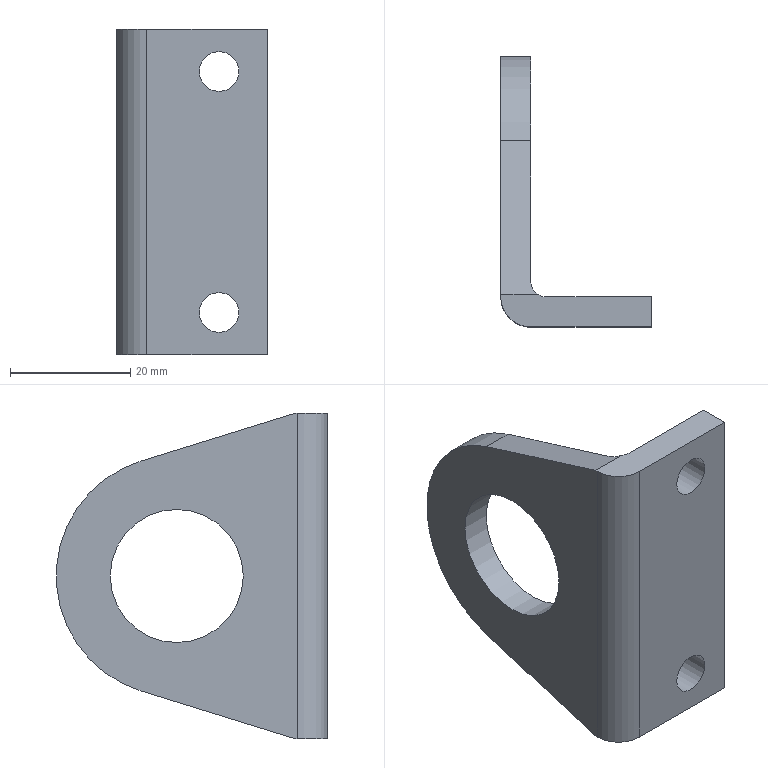Part | STEP file | 1_34 | 1 solid | 15 faces | box 25 x 45 x 54 mm | volume 12239 mm3 | plane 9 | cylinder 6 | commonest cylinder face diameters 6.6 x2 5 x1 10 x1 22.1 x1 40 x1
STEP:
#1=CARTESIAN_POINT('',(0.,0.,0.));
#2=DIRECTION('',(0.,0.,1.));
#3=DIRECTION('',(1.,0.,0.));
#4=AXIS2_PLACEMENT_3D('',#1,#2,#3);
#5=CARTESIAN_POINT('',(5.,25.,11.05));
#6=VERTEX_POINT('',#5);
#7=CARTESIAN_POINT('',(5.,25.,0.));
#8=DIRECTION('',(1.,0.,0.));
#9=DIRECTION('',(0.,1.,0.));
#10=AXIS2_PLACEMENT_3D('',#7,#8,#9);
#11=CIRCLE('',#10,11.05);
#12=CARTESIAN_POINT('',(5.1,25.,0.));
#13=DIRECTION('',(1.,0.,0.));
#14=DIRECTION('',(0.,0.,1.));
#15=AXIS2_PLACEMENT_3D('',#12,#13,#14);
#16=CYLINDRICAL_SURFACE('',#15,11.05);
#17=CARTESIAN_POINT('',(-1.571,-0.1));
#18=DIRECTION('',(1.,0.));
#19=VECTOR('',#18,1.);
#20=LINE('',#17,#19);
#21=(GEOMETRIC_REPRESENTATION_CONTEXT(2)PARAMETRIC_REPRESENTATION_CONTEXT()REPRESENTATION_CONTEXT('',''));
#22=DEFINITIONAL_REPRESENTATION('',(#20),#21);
#23=PCURVE('',#16,#22);
#24=CARTESIAN_POINT('',(5.,7.5,27.));
#25=DIRECTION('',(1.,0.,0.));
#26=DIRECTION('',(0.,0.,-1.));
#27=AXIS2_PLACEMENT_3D('',#24,#25,#26);
#28=PLANE('',#27);
#29=CARTESIAN_POINT('',(27.,17.5));
#30=DIRECTION('',(0.,1.));
#31=AXIS2_PLACEMENT_2D('',#29,#30);
#32=CIRCLE('',#31,11.05);
#33=(GEOMETRIC_REPRESENTATION_CONTEXT(2)PARAMETRIC_REPRESENTATION_CONTEXT()REPRESENTATION_CONTEXT('',''));
#34=DEFINITIONAL_REPRESENTATION('',(#32),#33);
#35=PCURVE('',#28,#34);
#36=SURFACE_CURVE('',#11,(#23,#35),.PCURVE_S1.);
#37=EDGE_CURVE('',#6,#6,#36,.T.);
#38=ORIENTED_EDGE('',*,*,#37,.F.);
#39=CARTESIAN_POINT('',(0.,25.,11.05));
#40=VERTEX_POINT('',#39);
#41=CARTESIAN_POINT('',(0.,25.,11.05));
#42=CARTESIAN_POINT('',(5.,25.,11.05));
#43=B_SPLINE_CURVE_WITH_KNOTS('',1,(#41,#42),.UNSPECIFIED.,.F.,.F.,(2,2),(-5.1,-0.1),.PIECEWISE_BEZIER_KNOTS.);
#44=CARTESIAN_POINT('',(0.,0.));
#45=DIRECTION('',(0.,1.));
#46=VECTOR('',#45,1.);
#47=LINE('',#44,#46);
#48=(GEOMETRIC_REPRESENTATION_CONTEXT(2)PARAMETRIC_REPRESENTATION_CONTEXT()REPRESENTATION_CONTEXT('',''));
#49=DEFINITIONAL_REPRESENTATION('',(#47),#48);
#50=PCURVE('',#16,#49);
#51=CARTESIAN_POINT('',(6.283,0.));
#52=DIRECTION('',(0.,1.));
#53=VECTOR('',#52,1.);
#54=LINE('',#51,#53);
#55=(GEOMETRIC_REPRESENTATION_CONTEXT(2)PARAMETRIC_REPRESENTATION_CONTEXT()REPRESENTATION_CONTEXT('',''));
#56=DEFINITIONAL_REPRESENTATION('',(#54),#55);
#57=PCURVE('',#16,#56);
#58=SEAM_CURVE('',#43,(#50,#57),.PCURVE_S1.);
#59=EDGE_CURVE('',#40,#6,#58,.T.);
#60=ORIENTED_EDGE('',*,*,#59,.F.);
#61=CARTESIAN_POINT('',(0.,25.,0.));
#62=DIRECTION('',(1.,0.,0.));
#63=DIRECTION('',(0.,0.,-1.));
#64=AXIS2_PLACEMENT_3D('',#61,#62,#63);
#65=CIRCLE('',#64,11.05);
#66=CARTESIAN_POINT('',(-3.142,-5.1));
#67=DIRECTION('',(1.,0.));
#68=VECTOR('',#67,1.);
#69=LINE('',#66,#68);
#70=(GEOMETRIC_REPRESENTATION_CONTEXT(2)PARAMETRIC_REPRESENTATION_CONTEXT()REPRESENTATION_CONTEXT('',''));
#71=DEFINITIONAL_REPRESENTATION('',(#69),#70);
#72=PCURVE('',#16,#71);
#73=CARTESIAN_POINT('',(0.,50.,27.));
#74=DIRECTION('',(-1.,0.,0.));
#75=DIRECTION('',(0.,0.,1.));
#76=AXIS2_PLACEMENT_3D('',#73,#74,#75);
#77=PLANE('',#76);
#78=CARTESIAN_POINT('',(-38.05,-25.));
#79=CARTESIAN_POINT('',(-38.05,-5.861));
#80=CARTESIAN_POINT('',(-21.475,-15.43));
#81=CARTESIAN_POINT('',(-4.9,-25.));
#82=CARTESIAN_POINT('',(-21.475,-34.57));
#83=CARTESIAN_POINT('',(-38.05,-44.139));
#84=CARTESIAN_POINT('',(-38.05,-25.));
#85=(BOUNDED_CURVE()B_SPLINE_CURVE(2,(#78,#79,#80,#81,#82,#83,#84),.UNSPECIFIED.,.T.,.F.)B_SPLINE_CURVE_WITH_KNOTS((1,2,2,2,2,1),(-2.094,0.,2.094,4.189,6.283,8.378),.UNSPECIFIED.)CURVE()GEOMETRIC_REPRESENTATION_ITEM()RATIONAL_B_SPLINE_CURVE((1.,0.5,1.,0.5,1.,0.5,1.))REPRESENTATION_ITEM(''));
#86=(GEOMETRIC_REPRESENTATION_CONTEXT(2)PARAMETRIC_REPRESENTATION_CONTEXT()REPRESENTATION_CONTEXT('',''));
#87=DEFINITIONAL_REPRESENTATION('',(#85),#86);
#88=PCURVE('',#77,#87);
#89=SURFACE_CURVE('',#65,(#72,#88),.PCURVE_S1.);
#90=EDGE_CURVE('',#40,#40,#89,.T.);
#91=ORIENTED_EDGE('',*,*,#90,.T.);
#92=ORIENTED_EDGE('',*,*,#59,.T.);
#93=EDGE_LOOP('',(#38,#60,#91,#92));
#94=FACE_BOUND('',#93,.F.);
#95=ADVANCED_FACE('',(#94),#16,.F.);
#96=CARTESIAN_POINT('',(0.,5.423,27.));
#97=VERTEX_POINT('',#96);
#98=CARTESIAN_POINT('',(0.,30.917,19.105));
#99=VERTEX_POINT('',#98);
#100=CARTESIAN_POINT('',(0.,5.423,27.));
#101=DIRECTION('',(0.,0.9552,-0.2958));
#102=VECTOR('',#101,1.);
#103=LINE('',#100,#102);
#104=CARTESIAN_POINT('',(0.,-44.577));
#105=DIRECTION('',(-0.2958,0.9552));
#106=VECTOR('',#105,1.);
#107=LINE('',#104,#106);
#108=(GEOMETRIC_REPRESENTATION_CONTEXT(2)PARAMETRIC_REPRESENTATION_CONTEXT()REPRESENTATION_CONTEXT('',''));
#109=DEFINITIONAL_REPRESENTATION('',(#107),#108);
#110=PCURVE('',#77,#109);
#111=CARTESIAN_POINT('',(17.,-1.,28.989));
#112=DIRECTION('',(0.,-0.2958,-0.9552));
#113=DIRECTION('',(-1.,0.,0.));
#114=AXIS2_PLACEMENT_3D('',#111,#112,#113);
#115=PLANE('',#114);
#116=CARTESIAN_POINT('',(17.,6.724));
#117=DIRECTION('',(0.,1.));
#118=VECTOR('',#117,1.);
#119=LINE('',#116,#118);
#120=(GEOMETRIC_REPRESENTATION_CONTEXT(2)PARAMETRIC_REPRESENTATION_CONTEXT()REPRESENTATION_CONTEXT('',''));
#121=DEFINITIONAL_REPRESENTATION('',(#119),#120);
#122=PCURVE('',#115,#121);
#123=SURFACE_CURVE('',#103,(#110,#122),.PCURVE_S1.);
#124=EDGE_CURVE('',#97,#99,#123,.T.);
#125=ORIENTED_EDGE('',*,*,#124,.T.);
#126=CARTESIAN_POINT('',(0.,30.917,-19.105));
#127=VERTEX_POINT('',#126);
#128=CARTESIAN_POINT('',(0.,25.,0.));
#129=DIRECTION('',(-1.,0.,0.));
#130=DIRECTION('',(0.,1.,0.));
#131=AXIS2_PLACEMENT_3D('',#128,#129,#130);
#132=CIRCLE('',#131,20.);
#133=CARTESIAN_POINT('',(-27.,-25.));
#134=DIRECTION('',(0.,1.));
#135=AXIS2_PLACEMENT_2D('',#133,#134);
#136=CIRCLE('',#135,20.);
#137=(GEOMETRIC_REPRESENTATION_CONTEXT(2)PARAMETRIC_REPRESENTATION_CONTEXT()REPRESENTATION_CONTEXT('',''));
#138=DEFINITIONAL_REPRESENTATION('',(#136),#137);
#139=PCURVE('',#77,#138);
#140=CARTESIAN_POINT('',(17.,25.,0.));
#141=DIRECTION('',(1.,0.,0.));
#142=DIRECTION('',(0.,-0.2958,-0.9552));
#143=AXIS2_PLACEMENT_3D('',#140,#141,#142);
#144=CYLINDRICAL_SURFACE('',#143,20.);
#145=CARTESIAN_POINT('',(8.154,-17.));
#146=DIRECTION('',(-1.,0.));
#147=VECTOR('',#146,1.);
#148=LINE('',#145,#147);
#149=(GEOMETRIC_REPRESENTATION_CONTEXT(2)PARAMETRIC_REPRESENTATION_CONTEXT()REPRESENTATION_CONTEXT('',''));
#150=DEFINITIONAL_REPRESENTATION('',(#148),#149);
#151=PCURVE('',#144,#150);
#152=SURFACE_CURVE('',#132,(#139,#151),.PCURVE_S1.);
#153=EDGE_CURVE('',#99,#127,#152,.T.);
#154=ORIENTED_EDGE('',*,*,#153,.T.);
#155=CARTESIAN_POINT('',(0.,5.423,-27.));
#156=VERTEX_POINT('',#155);
#157=CARTESIAN_POINT('',(0.,30.917,-19.105));
#158=DIRECTION('',(0.,-0.9552,-0.2958));
#159=VECTOR('',#158,1.);
#160=LINE('',#157,#159);
#161=CARTESIAN_POINT('',(-46.105,-19.083));
#162=DIRECTION('',(-0.2958,-0.9552));
#163=VECTOR('',#162,1.);
#164=LINE('',#161,#163);
#165=(GEOMETRIC_REPRESENTATION_CONTEXT(2)PARAMETRIC_REPRESENTATION_CONTEXT()REPRESENTATION_CONTEXT('',''));
#166=DEFINITIONAL_REPRESENTATION('',(#164),#165);
#167=PCURVE('',#77,#166);
#168=CARTESIAN_POINT('',(17.,30.917,-19.105));
#169=DIRECTION('',(0.,-0.2958,0.9552));
#170=DIRECTION('',(1.,0.,0.));
#171=AXIS2_PLACEMENT_3D('',#168,#169,#170);
#172=PLANE('',#171);
#173=CARTESIAN_POINT('',(-17.,0.));
#174=DIRECTION('',(0.,-1.));
#175=VECTOR('',#174,1.);
#176=LINE('',#173,#175);
#177=(GEOMETRIC_REPRESENTATION_CONTEXT(2)PARAMETRIC_REPRESENTATION_CONTEXT()REPRESENTATION_CONTEXT('',''));
#178=DEFINITIONAL_REPRESENTATION('',(#176),#177);
#179=PCURVE('',#172,#178);
#180=SURFACE_CURVE('',#160,(#167,#179),.PCURVE_S1.);
#181=EDGE_CURVE('',#127,#156,#180,.T.);
#182=ORIENTED_EDGE('',*,*,#181,.T.);
#183=CARTESIAN_POINT('',(0.,5.,-27.));
#184=VERTEX_POINT('',#183);
#185=CARTESIAN_POINT('',(0.,5.423,-27.));
#186=DIRECTION('',(0.,-1.,0.));
#187=VECTOR('',#186,1.);
#188=LINE('',#185,#187);
#189=CARTESIAN_POINT('',(-54.,-44.577));
#190=DIRECTION('',(0.,-1.));
#191=VECTOR('',#190,1.);
#192=LINE('',#189,#191);
#193=(GEOMETRIC_REPRESENTATION_CONTEXT(2)PARAMETRIC_REPRESENTATION_CONTEXT()REPRESENTATION_CONTEXT('',''));
#194=DEFINITIONAL_REPRESENTATION('',(#192),#193);
#195=PCURVE('',#77,#194);
#196=CARTESIAN_POINT('',(0.,0.,-27.));
#197=DIRECTION('',(0.,0.,1.));
#198=DIRECTION('',(1.,0.,0.));
#199=AXIS2_PLACEMENT_3D('',#196,#197,#198);
#200=PLANE('',#199);
#201=CARTESIAN_POINT('',(0.,5.423));
#202=DIRECTION('',(0.,-1.));
#203=VECTOR('',#202,1.);
#204=LINE('',#201,#203);
#205=(GEOMETRIC_REPRESENTATION_CONTEXT(2)PARAMETRIC_REPRESENTATION_CONTEXT()REPRESENTATION_CONTEXT('',''));
#206=DEFINITIONAL_REPRESENTATION('',(#204),#205);
#207=PCURVE('',#200,#206);
#208=SURFACE_CURVE('',#188,(#195,#207),.PCURVE_S1.);
#209=EDGE_CURVE('',#156,#184,#208,.T.);
#210=ORIENTED_EDGE('',*,*,#209,.T.);
#211=CARTESIAN_POINT('',(0.,5.,27.));
#212=VERTEX_POINT('',#211);
#213=CARTESIAN_POINT('',(0.,5.,27.));
#214=DIRECTION('',(0.,0.,-1.));
#215=VECTOR('',#214,1.);
#216=LINE('',#213,#215);
#217=CARTESIAN_POINT('',(0.,-45.));
#218=DIRECTION('',(-1.,0.));
#219=VECTOR('',#218,1.);
#220=LINE('',#217,#219);
#221=(GEOMETRIC_REPRESENTATION_CONTEXT(2)PARAMETRIC_REPRESENTATION_CONTEXT()REPRESENTATION_CONTEXT('',''));
#222=DEFINITIONAL_REPRESENTATION('',(#220),#221);
#223=PCURVE('',#77,#222);
#224=CARTESIAN_POINT('',(5.,5.,27.));
#225=DIRECTION('',(0.,0.,1.));
#226=DIRECTION('',(-1.,0.,0.));
#227=AXIS2_PLACEMENT_3D('',#224,#225,#226);
#228=CYLINDRICAL_SURFACE('',#227,5.);
#229=CARTESIAN_POINT('',(0.,0.));
#230=DIRECTION('',(0.,-1.));
#231=VECTOR('',#230,1.);
#232=LINE('',#229,#231);
#233=(GEOMETRIC_REPRESENTATION_CONTEXT(2)PARAMETRIC_REPRESENTATION_CONTEXT()REPRESENTATION_CONTEXT('',''));
#234=DEFINITIONAL_REPRESENTATION('',(#232),#233);
#235=PCURVE('',#228,#234);
#236=SURFACE_CURVE('',#216,(#223,#235),.PCURVE_S1.);
#237=EDGE_CURVE('',#212,#184,#236,.T.);
#238=ORIENTED_EDGE('',*,*,#237,.F.);
#239=CARTESIAN_POINT('',(0.,5.423,27.));
#240=DIRECTION('',(0.,-1.,0.));
#241=VECTOR('',#240,1.);
#242=LINE('',#239,#241);
#243=CARTESIAN_POINT('',(0.,-44.577));
#244=DIRECTION('',(0.,-1.));
#245=VECTOR('',#244,1.);
#246=LINE('',#243,#245);
#247=(GEOMETRIC_REPRESENTATION_CONTEXT(2)PARAMETRIC_REPRESENTATION_CONTEXT()REPRESENTATION_CONTEXT('',''));
#248=DEFINITIONAL_REPRESENTATION('',(#246),#247);
#249=PCURVE('',#77,#248);
#250=CARTESIAN_POINT('',(0.,0.,27.));
#251=DIRECTION('',(0.,0.,1.));
#252=DIRECTION('',(1.,0.,0.));
#253=AXIS2_PLACEMENT_3D('',#250,#251,#252);
#254=PLANE('',#253);
#255=CARTESIAN_POINT('',(0.,5.423));
#256=DIRECTION('',(0.,-1.));
#257=VECTOR('',#256,1.);
#258=LINE('',#255,#257);
#259=(GEOMETRIC_REPRESENTATION_CONTEXT(2)PARAMETRIC_REPRESENTATION_CONTEXT()REPRESENTATION_CONTEXT('',''));
#260=DEFINITIONAL_REPRESENTATION('',(#258),#259);
#261=PCURVE('',#254,#260);
#262=SURFACE_CURVE('',#242,(#249,#261),.PCURVE_S1.);
#263=EDGE_CURVE('',#97,#212,#262,.T.);
#264=ORIENTED_EDGE('',*,*,#263,.F.);
#265=EDGE_LOOP('',(#125,#154,#182,#210,#238,#264));
#266=FACE_BOUND('',#265,.T.);
#267=ORIENTED_EDGE('',*,*,#90,.T.);
#268=EDGE_LOOP('',(#267));
#269=FACE_BOUND('',#268,.T.);
#270=ADVANCED_FACE('',(#266,#269),#77,.T.);
#271=CARTESIAN_POINT('',(5.,30.917,19.105));
#272=VERTEX_POINT('',#271);
#273=CARTESIAN_POINT('',(5.,7.5,26.357));
#274=VERTEX_POINT('',#273);
#275=CARTESIAN_POINT('',(5.,30.917,19.105));
#276=DIRECTION('',(0.,-0.9552,0.2958));
#277=VECTOR('',#276,1.);
#278=LINE('',#275,#277);
#279=CARTESIAN_POINT('',(7.895,23.417));
#280=DIRECTION('',(-0.2958,-0.9552));
#281=VECTOR('',#280,1.);
#282=LINE('',#279,#281);
#283=(GEOMETRIC_REPRESENTATION_CONTEXT(2)PARAMETRIC_REPRESENTATION_CONTEXT()REPRESENTATION_CONTEXT('',''));
#284=DEFINITIONAL_REPRESENTATION('',(#282),#283);
#285=PCURVE('',#28,#284);
#286=CARTESIAN_POINT('',(12.,33.412));
#287=DIRECTION('',(0.,-1.));
#288=VECTOR('',#287,1.);
#289=LINE('',#286,#288);
#290=(GEOMETRIC_REPRESENTATION_CONTEXT(2)PARAMETRIC_REPRESENTATION_CONTEXT()REPRESENTATION_CONTEXT('',''));
#291=DEFINITIONAL_REPRESENTATION('',(#289),#290);
#292=PCURVE('',#115,#291);
#293=SURFACE_CURVE('',#278,(#285,#292),.PCURVE_S1.);
#294=EDGE_CURVE('',#272,#274,#293,.T.);
#295=ORIENTED_EDGE('',*,*,#294,.T.);
#296=CARTESIAN_POINT('',(5.,7.5,-26.357));
#297=VERTEX_POINT('',#296);
#298=CARTESIAN_POINT('',(5.,7.5,26.357));
#299=DIRECTION('',(0.,0.,-1.));
#300=VECTOR('',#299,1.);
#301=LINE('',#298,#300);
#302=CARTESIAN_POINT('',(0.6433,0.));
#303=DIRECTION('',(1.,0.));
#304=VECTOR('',#303,1.);
#305=LINE('',#302,#304);
#306=(GEOMETRIC_REPRESENTATION_CONTEXT(2)PARAMETRIC_REPRESENTATION_CONTEXT()REPRESENTATION_CONTEXT('',''));
#307=DEFINITIONAL_REPRESENTATION('',(#305),#306);
#308=PCURVE('',#28,#307);
#309=CARTESIAN_POINT('',(7.5,7.5,27.));
#310=DIRECTION('',(0.,0.,1.));
#311=DIRECTION('',(0.,1.,0.));
#312=AXIS2_PLACEMENT_3D('',#309,#310,#311);
#313=CYLINDRICAL_SURFACE('',#312,2.5);
#314=CARTESIAN_POINT('',(1.571,-0.6433));
#315=DIRECTION('',(0.,-1.));
#316=VECTOR('',#315,1.);
#317=LINE('',#314,#316);
#318=(GEOMETRIC_REPRESENTATION_CONTEXT(2)PARAMETRIC_REPRESENTATION_CONTEXT()REPRESENTATION_CONTEXT('',''));
#319=DEFINITIONAL_REPRESENTATION('',(#317),#318);
#320=PCURVE('',#313,#319);
#321=SURFACE_CURVE('',#301,(#308,#320),.PCURVE_S1.);
#322=EDGE_CURVE('',#274,#297,#321,.T.);
#323=ORIENTED_EDGE('',*,*,#322,.T.);
#324=CARTESIAN_POINT('',(5.,30.917,-19.105));
#325=VERTEX_POINT('',#324);
#326=CARTESIAN_POINT('',(5.,7.5,-26.357));
#327=DIRECTION('',(0.,0.9552,0.2958));
#328=VECTOR('',#327,1.);
#329=LINE('',#326,#328);
#330=CARTESIAN_POINT('',(53.357,-0.000000001));
#331=DIRECTION('',(-0.2958,0.9552));
#332=VECTOR('',#331,1.);
#333=LINE('',#330,#332);
#334=(GEOMETRIC_REPRESENTATION_CONTEXT(2)PARAMETRIC_REPRESENTATION_CONTEXT()REPRESENTATION_CONTEXT('',''));
#335=DEFINITIONAL_REPRESENTATION('',(#333),#334);
#336=PCURVE('',#28,#335);
#337=CARTESIAN_POINT('',(-12.,-24.514));
#338=DIRECTION('',(0.,1.));
#339=VECTOR('',#338,1.);
#340=LINE('',#337,#339);
#341=(GEOMETRIC_REPRESENTATION_CONTEXT(2)PARAMETRIC_REPRESENTATION_CONTEXT()REPRESENTATION_CONTEXT('',''));
#342=DEFINITIONAL_REPRESENTATION('',(#340),#341);
#343=PCURVE('',#172,#342);
#344=SURFACE_CURVE('',#329,(#336,#343),.PCURVE_S1.);
#345=EDGE_CURVE('',#297,#325,#344,.T.);
#346=ORIENTED_EDGE('',*,*,#345,.T.);
#347=CARTESIAN_POINT('',(5.,25.,0.));
#348=DIRECTION('',(1.,0.,0.));
#349=DIRECTION('',(0.,1.,0.));
#350=AXIS2_PLACEMENT_3D('',#347,#348,#349);
#351=CIRCLE('',#350,20.);
#352=CARTESIAN_POINT('',(27.,17.5));
#353=DIRECTION('',(0.,1.));
#354=AXIS2_PLACEMENT_2D('',#352,#353);
#355=CIRCLE('',#354,20.);
#356=(GEOMETRIC_REPRESENTATION_CONTEXT(2)PARAMETRIC_REPRESENTATION_CONTEXT()REPRESENTATION_CONTEXT('',''));
#357=DEFINITIONAL_REPRESENTATION('',(#355),#356);
#358=PCURVE('',#28,#357);
#359=CARTESIAN_POINT('',(-4.412,-12.));
#360=DIRECTION('',(1.,0.));
#361=VECTOR('',#360,1.);
#362=LINE('',#359,#361);
#363=(GEOMETRIC_REPRESENTATION_CONTEXT(2)PARAMETRIC_REPRESENTATION_CONTEXT()REPRESENTATION_CONTEXT('',''));
#364=DEFINITIONAL_REPRESENTATION('',(#362),#363);
#365=PCURVE('',#144,#364);
#366=SURFACE_CURVE('',#351,(#358,#365),.PCURVE_S1.);
#367=EDGE_CURVE('',#325,#272,#366,.T.);
#368=ORIENTED_EDGE('',*,*,#367,.T.);
#369=EDGE_LOOP('',(#295,#323,#346,#368));
#370=FACE_BOUND('',#369,.T.);
#371=ORIENTED_EDGE('',*,*,#37,.F.);
#372=EDGE_LOOP('',(#371));
#373=FACE_BOUND('',#372,.T.);
#374=ADVANCED_FACE('',(#370,#373),#28,.T.);
#375=ORIENTED_EDGE('',*,*,#124,.F.);
#376=CARTESIAN_POINT('',(6.109,5.423,27.));
#377=VERTEX_POINT('',#376);
#378=CARTESIAN_POINT('',(6.109,5.423,27.));
#379=DIRECTION('',(-1.,0.,0.));
#380=VECTOR('',#379,1.);
#381=LINE('',#378,#380);
#382=CARTESIAN_POINT('',(10.891,6.724));
#383=DIRECTION('',(1.,0.));
#384=VECTOR('',#383,1.);
#385=LINE('',#382,#384);
#386=(GEOMETRIC_REPRESENTATION_CONTEXT(2)PARAMETRIC_REPRESENTATION_CONTEXT()REPRESENTATION_CONTEXT('',''));
#387=DEFINITIONAL_REPRESENTATION('',(#385),#386);
#388=PCURVE('',#115,#387);
#389=CARTESIAN_POINT('',(6.109,5.423));
#390=DIRECTION('',(-1.,0.));
#391=VECTOR('',#390,1.);
#392=LINE('',#389,#391);
#393=(GEOMETRIC_REPRESENTATION_CONTEXT(2)PARAMETRIC_REPRESENTATION_CONTEXT()REPRESENTATION_CONTEXT('',''));
#394=DEFINITIONAL_REPRESENTATION('',(#392),#393);
#395=PCURVE('',#254,#394);
#396=SURFACE_CURVE('',#381,(#388,#395),.PCURVE_S1.);
#397=EDGE_CURVE('',#377,#97,#396,.T.);
#398=ORIENTED_EDGE('',*,*,#397,.F.);
#399=CARTESIAN_POINT('',(7.5,7.5,26.357));
#400=DIRECTION('',(0.,0.2958,0.9552));
#401=DIRECTION('',(-0.0009461,-0.9552,0.2958));
#402=AXIS2_PLACEMENT_3D('',#399,#400,#401);
#403=ELLIPSE('',#402,2.617,2.5);
#404=CARTESIAN_POINT('',(9.502,6.281));
#405=CARTESIAN_POINT('',(5.171,6.277));
#406=CARTESIAN_POINT('',(7.333,10.205));
#407=CARTESIAN_POINT('',(9.495,14.133));
#408=CARTESIAN_POINT('',(11.664,10.209));
#409=CARTESIAN_POINT('',(13.833,6.285));
#410=CARTESIAN_POINT('',(9.502,6.281));
#411=(BOUNDED_CURVE()B_SPLINE_CURVE(2,(#404,#405,#406,#407,#408,#409,#410),.UNSPECIFIED.,.T.,.F.)B_SPLINE_CURVE_WITH_KNOTS((1,2,2,2,2,1),(-2.094,0.,2.094,4.189,6.283,8.378),.UNSPECIFIED.)CURVE()GEOMETRIC_REPRESENTATION_ITEM()RATIONAL_B_SPLINE_CURVE((1.,0.5,1.,0.5,1.,0.5,1.))REPRESENTATION_ITEM(''));
#412=(GEOMETRIC_REPRESENTATION_CONTEXT(2)PARAMETRIC_REPRESENTATION_CONTEXT()REPRESENTATION_CONTEXT('',''));
#413=DEFINITIONAL_REPRESENTATION('',(#411),#412);
#414=PCURVE('',#115,#413);
#415=CARTESIAN_POINT('',(1.571,-0.6433));
#416=CARTESIAN_POINT('',(1.586,-0.6318));
#417=CARTESIAN_POINT('',(1.615,-0.6087));
#418=CARTESIAN_POINT('',(1.66,-0.5743));
#419=CARTESIAN_POINT('',(1.705,-0.54));
#420=CARTESIAN_POINT('',(1.749,-0.5059));
#421=CARTESIAN_POINT('',(1.794,-0.4721));
#422=CARTESIAN_POINT('',(1.838,-0.4386));
#423=CARTESIAN_POINT('',(1.883,-0.4055));
#424=CARTESIAN_POINT('',(1.927,-0.3729));
#425=CARTESIAN_POINT('',(1.972,-0.3408));
#426=CARTESIAN_POINT('',(2.017,-0.3094));
#427=CARTESIAN_POINT('',(2.061,-0.2786));
#428=CARTESIAN_POINT('',(2.106,-0.2485));
#429=CARTESIAN_POINT('',(2.15,-0.2192));
#430=CARTESIAN_POINT('',(2.195,-0.1907));
#431=CARTESIAN_POINT('',(2.239,-0.1632));
#432=CARTESIAN_POINT('',(2.284,-0.1366));
#433=CARTESIAN_POINT('',(2.329,-0.111));
#434=CARTESIAN_POINT('',(2.373,-0.08643));
#435=CARTESIAN_POINT('',(2.418,-0.06299));
#436=CARTESIAN_POINT('',(2.462,-0.04071));
#437=CARTESIAN_POINT('',(2.507,-0.01963));
#438=CARTESIAN_POINT('',(2.537,-0.006402));
#439=CARTESIAN_POINT('',(2.551,0.));
#440=B_SPLINE_CURVE_WITH_KNOTS('',3,(#415,#416,#417,#418,#419,#420,#421,#422,#423,#424,#425,#426,#427,#428,#429,#430,#431,#432,#433,#434,#435,#436,#437,#438,#439),.UNSPECIFIED.,.F.,.F.,(4,1,1,1,1,1,1,1,1,1,1,1,1,1,1,1,1,1,1,1,1,1,4),(4.713,4.758,4.803,4.847,4.892,4.936,4.981,5.025,5.07,5.115,5.159,5.204,5.248,5.293,5.337,5.382,5.426,5.471,5.516,5.56,5.605,5.649,5.694),.QUASI_UNIFORM_KNOTS.);
#441=(GEOMETRIC_REPRESENTATION_CONTEXT(2)PARAMETRIC_REPRESENTATION_CONTEXT()REPRESENTATION_CONTEXT('',''));
#442=DEFINITIONAL_REPRESENTATION('',(#440),#441);
#443=PCURVE('',#313,#442);
#444=SURFACE_CURVE('',#403,(#414,#443),.PCURVE_S1.);
#445=EDGE_CURVE('',#274,#377,#444,.T.);
#446=ORIENTED_EDGE('',*,*,#445,.F.);
#447=ORIENTED_EDGE('',*,*,#294,.F.);
#448=CARTESIAN_POINT('',(5.,30.917,19.105));
#449=DIRECTION('',(-1.,0.,0.));
#450=VECTOR('',#449,1.);
#451=LINE('',#448,#450);
#452=CARTESIAN_POINT('',(12.,33.412));
#453=DIRECTION('',(1.,0.));
#454=VECTOR('',#453,1.);
#455=LINE('',#452,#454);
#456=(GEOMETRIC_REPRESENTATION_CONTEXT(2)PARAMETRIC_REPRESENTATION_CONTEXT()REPRESENTATION_CONTEXT('',''));
#457=DEFINITIONAL_REPRESENTATION('',(#455),#456);
#458=PCURVE('',#115,#457);
#459=CARTESIAN_POINT('',(3.142,-12.));
#460=DIRECTION('',(0.,-1.));
#461=VECTOR('',#460,1.);
#462=LINE('',#459,#461);
#463=(GEOMETRIC_REPRESENTATION_CONTEXT(2)PARAMETRIC_REPRESENTATION_CONTEXT()REPRESENTATION_CONTEXT('',''));
#464=DEFINITIONAL_REPRESENTATION('',(#462),#463);
#465=PCURVE('',#144,#464);
#466=SURFACE_CURVE('',#451,(#458,#465),.PCURVE_S1.);
#467=EDGE_CURVE('',#272,#99,#466,.T.);
#468=ORIENTED_EDGE('',*,*,#467,.T.);
#469=EDGE_LOOP('',(#375,#398,#446,#447,#468));
#470=FACE_BOUND('',#469,.T.);
#471=ADVANCED_FACE('',(#470),#115,.F.);
#472=ORIENTED_EDGE('',*,*,#153,.F.);
#473=ORIENTED_EDGE('',*,*,#467,.F.);
#474=ORIENTED_EDGE('',*,*,#367,.F.);
#475=CARTESIAN_POINT('',(0.,30.917,-19.105));
#476=DIRECTION('',(1.,0.,0.));
#477=VECTOR('',#476,1.);
#478=LINE('',#475,#477);
#479=CARTESIAN_POINT('',(0.6006,-17.));
#480=DIRECTION('',(0.,1.));
#481=VECTOR('',#480,1.);
#482=LINE('',#479,#481);
#483=(GEOMETRIC_REPRESENTATION_CONTEXT(2)PARAMETRIC_REPRESENTATION_CONTEXT()REPRESENTATION_CONTEXT('',''));
#484=DEFINITIONAL_REPRESENTATION('',(#482),#483);
#485=PCURVE('',#144,#484);
#486=CARTESIAN_POINT('',(-17.,0.));
#487=DIRECTION('',(1.,0.));
#488=VECTOR('',#487,1.);
#489=LINE('',#486,#488);
#490=(GEOMETRIC_REPRESENTATION_CONTEXT(2)PARAMETRIC_REPRESENTATION_CONTEXT()REPRESENTATION_CONTEXT('',''));
#491=DEFINITIONAL_REPRESENTATION('',(#489),#490);
#492=PCURVE('',#172,#491);
#493=SURFACE_CURVE('',#478,(#485,#492),.PCURVE_S1.);
#494=EDGE_CURVE('',#127,#325,#493,.T.);
#495=ORIENTED_EDGE('',*,*,#494,.F.);
#496=EDGE_LOOP('',(#472,#473,#474,#495));
#497=FACE_BOUND('',#496,.T.);
#498=ADVANCED_FACE('',(#497),#144,.T.);
#499=ORIENTED_EDGE('',*,*,#181,.F.);
#500=ORIENTED_EDGE('',*,*,#494,.T.);
#501=ORIENTED_EDGE('',*,*,#345,.F.);
#502=CARTESIAN_POINT('',(6.109,5.423,-27.));
#503=VERTEX_POINT('',#502);
#504=CARTESIAN_POINT('',(7.5,7.5,-26.357));
#505=DIRECTION('',(0.,0.2958,-0.9552));
#506=DIRECTION('',(0.0005678,0.9552,0.2958));
#507=AXIS2_PLACEMENT_3D('',#504,#505,#506);
#508=ELLIPSE('',#507,2.617,2.5);
#509=CARTESIAN_POINT('',(-9.498,-21.896));
#510=CARTESIAN_POINT('',(-5.167,-21.899));
#511=CARTESIAN_POINT('',(-7.335,-25.824));
#512=CARTESIAN_POINT('',(-9.503,-29.748));
#513=CARTESIAN_POINT('',(-11.666,-25.821));
#514=CARTESIAN_POINT('',(-13.829,-21.894));
#515=CARTESIAN_POINT('',(-9.498,-21.896));
#516=(BOUNDED_CURVE()B_SPLINE_CURVE(2,(#509,#510,#511,#512,#513,#514,#515),.UNSPECIFIED.,.T.,.F.)B_SPLINE_CURVE_WITH_KNOTS((1,2,2,2,2,1),(-2.094,0.,2.094,4.189,6.283,8.378),.UNSPECIFIED.)CURVE()GEOMETRIC_REPRESENTATION_ITEM()RATIONAL_B_SPLINE_CURVE((1.,0.5,1.,0.5,1.,0.5,1.))REPRESENTATION_ITEM(''));
#517=(GEOMETRIC_REPRESENTATION_CONTEXT(2)PARAMETRIC_REPRESENTATION_CONTEXT()REPRESENTATION_CONTEXT('',''));
#518=DEFINITIONAL_REPRESENTATION('',(#516),#517);
#519=PCURVE('',#172,#518);
#520=CARTESIAN_POINT('',(2.551,-54.));
#521=CARTESIAN_POINT('',(2.537,-53.994));
#522=CARTESIAN_POINT('',(2.507,-53.98));
#523=CARTESIAN_POINT('',(2.462,-53.959));
#524=CARTESIAN_POINT('',(2.418,-53.937));
#525=CARTESIAN_POINT('',(2.373,-53.914));
#526=CARTESIAN_POINT('',(2.329,-53.889));
#527=CARTESIAN_POINT('',(2.284,-53.863));
#528=CARTESIAN_POINT('',(2.239,-53.837));
#529=CARTESIAN_POINT('',(2.195,-53.809));
#530=CARTESIAN_POINT('',(2.15,-53.781));
#531=CARTESIAN_POINT('',(2.106,-53.752));
#532=CARTESIAN_POINT('',(2.061,-53.721));
#533=CARTESIAN_POINT('',(2.017,-53.691));
#534=CARTESIAN_POINT('',(1.972,-53.659));
#535=CARTESIAN_POINT('',(1.927,-53.627));
#536=CARTESIAN_POINT('',(1.883,-53.594));
#537=CARTESIAN_POINT('',(1.838,-53.561));
#538=CARTESIAN_POINT('',(1.794,-53.528));
#539=CARTESIAN_POINT('',(1.749,-53.494));
#540=CARTESIAN_POINT('',(1.705,-53.46));
#541=CARTESIAN_POINT('',(1.66,-53.426));
#542=CARTESIAN_POINT('',(1.615,-53.391));
#543=CARTESIAN_POINT('',(1.586,-53.368));
#544=CARTESIAN_POINT('',(1.571,-53.357));
#545=B_SPLINE_CURVE_WITH_KNOTS('',3,(#520,#521,#522,#523,#524,#525,#526,#527,#528,#529,#530,#531,#532,#533,#534,#535,#536,#537,#538,#539,#540,#541,#542,#543,#544),.UNSPECIFIED.,.F.,.F.,(4,1,1,1,1,1,1,1,1,1,1,1,1,1,1,1,1,1,1,1,1,1,4),(3.731,3.776,3.82,3.865,3.91,3.954,3.999,4.043,4.088,4.132,4.177,4.222,4.266,4.311,4.355,4.4,4.444,4.489,4.534,4.578,4.623,4.667,4.712),.QUASI_UNIFORM_KNOTS.);
#546=(GEOMETRIC_REPRESENTATION_CONTEXT(2)PARAMETRIC_REPRESENTATION_CONTEXT()REPRESENTATION_CONTEXT('',''));
#547=DEFINITIONAL_REPRESENTATION('',(#545),#546);
#548=PCURVE('',#313,#547);
#549=SURFACE_CURVE('',#508,(#519,#548),.PCURVE_S1.);
#550=EDGE_CURVE('',#503,#297,#549,.T.);
#551=ORIENTED_EDGE('',*,*,#550,.F.);
#552=CARTESIAN_POINT('',(0.,5.423,-27.));
#553=DIRECTION('',(1.,0.,0.));
#554=VECTOR('',#553,1.);
#555=LINE('',#552,#554);
#556=CARTESIAN_POINT('',(-17.,-26.688));
#557=DIRECTION('',(1.,0.));
#558=VECTOR('',#557,1.);
#559=LINE('',#556,#558);
#560=(GEOMETRIC_REPRESENTATION_CONTEXT(2)PARAMETRIC_REPRESENTATION_CONTEXT()REPRESENTATION_CONTEXT('',''));
#561=DEFINITIONAL_REPRESENTATION('',(#559),#560);
#562=PCURVE('',#172,#561);
#563=CARTESIAN_POINT('',(0.,5.423));
#564=DIRECTION('',(1.,0.));
#565=VECTOR('',#564,1.);
#566=LINE('',#563,#565);
#567=(GEOMETRIC_REPRESENTATION_CONTEXT(2)PARAMETRIC_REPRESENTATION_CONTEXT()REPRESENTATION_CONTEXT('',''));
#568=DEFINITIONAL_REPRESENTATION('',(#566),#567);
#569=PCURVE('',#200,#568);
#570=SURFACE_CURVE('',#555,(#562,#569),.PCURVE_S1.);
#571=EDGE_CURVE('',#156,#503,#570,.T.);
#572=ORIENTED_EDGE('',*,*,#571,.F.);
#573=EDGE_LOOP('',(#499,#500,#501,#551,#572));
#574=FACE_BOUND('',#573,.T.);
#575=ADVANCED_FACE('',(#574),#172,.F.);
#576=ORIENTED_EDGE('',*,*,#571,.T.);
#577=CARTESIAN_POINT('',(7.5,5.,-27.));
#578=VERTEX_POINT('',#577);
#579=CARTESIAN_POINT('',(7.5,7.5,-27.));
#580=DIRECTION('',(0.,0.,-1.));
#581=DIRECTION('',(-0.5565,-0.8308,0.));
#582=AXIS2_PLACEMENT_3D('',#579,#580,#581);
#583=CIRCLE('',#582,2.5);
#584=CARTESIAN_POINT('',(6.109,5.423));
#585=CARTESIAN_POINT('',(2.511,7.833));
#586=CARTESIAN_POINT('',(6.397,9.743));
#587=CARTESIAN_POINT('',(10.283,11.654));
#588=CARTESIAN_POINT('',(9.994,7.334));
#589=CARTESIAN_POINT('',(9.706,3.013));
#590=CARTESIAN_POINT('',(6.109,5.423));
#591=(BOUNDED_CURVE()B_SPLINE_CURVE(2,(#584,#585,#586,#587,#588,#589,#590),.UNSPECIFIED.,.T.,.F.)B_SPLINE_CURVE_WITH_KNOTS((1,2,2,2,2,1),(-2.094,0.,2.094,4.189,6.283,8.378),.UNSPECIFIED.)CURVE()GEOMETRIC_REPRESENTATION_ITEM()RATIONAL_B_SPLINE_CURVE((1.,0.5,1.,0.5,1.,0.5,1.))REPRESENTATION_ITEM(''));
#592=(GEOMETRIC_REPRESENTATION_CONTEXT(2)PARAMETRIC_REPRESENTATION_CONTEXT()REPRESENTATION_CONTEXT('',''));
#593=DEFINITIONAL_REPRESENTATION('',(#591),#592);
#594=PCURVE('',#200,#593);
#595=CARTESIAN_POINT('',(8.835,-54.));
#596=DIRECTION('',(-1.,0.));
#597=VECTOR('',#596,1.);
#598=LINE('',#595,#597);
#599=(GEOMETRIC_REPRESENTATION_CONTEXT(2)PARAMETRIC_REPRESENTATION_CONTEXT()REPRESENTATION_CONTEXT('',''));
#600=DEFINITIONAL_REPRESENTATION('',(#598),#599);
#601=PCURVE('',#313,#600);
#602=SURFACE_CURVE('',#583,(#594,#601),.PCURVE_S1.);
#603=EDGE_CURVE('',#578,#503,#602,.T.);
#604=ORIENTED_EDGE('',*,*,#603,.F.);
#605=CARTESIAN_POINT('',(25.,5.,-27.));
#606=VERTEX_POINT('',#605);
#607=CARTESIAN_POINT('',(25.,5.,-27.));
#608=DIRECTION('',(-1.,0.,0.));
#609=VECTOR('',#608,1.);
#610=LINE('',#607,#609);
#611=CARTESIAN_POINT('',(25.,5.));
#612=DIRECTION('',(-1.,0.));
#613=VECTOR('',#612,1.);
#614=LINE('',#611,#613);
#615=(GEOMETRIC_REPRESENTATION_CONTEXT(2)PARAMETRIC_REPRESENTATION_CONTEXT()REPRESENTATION_CONTEXT('',''));
#616=DEFINITIONAL_REPRESENTATION('',(#614),#615);
#617=PCURVE('',#200,#616);
#618=CARTESIAN_POINT('',(25.,5.,27.));
#619=DIRECTION('',(0.,1.,0.));
#620=DIRECTION('',(0.,0.,1.));
#621=AXIS2_PLACEMENT_3D('',#618,#619,#620);
#622=PLANE('',#621);
#623=CARTESIAN_POINT('',(-54.,0.));
#624=DIRECTION('',(0.,-1.));
#625=VECTOR('',#624,1.);
#626=LINE('',#623,#625);
#627=(GEOMETRIC_REPRESENTATION_CONTEXT(2)PARAMETRIC_REPRESENTATION_CONTEXT()REPRESENTATION_CONTEXT('',''));
#628=DEFINITIONAL_REPRESENTATION('',(#626),#627);
#629=PCURVE('',#622,#628);
#630=SURFACE_CURVE('',#610,(#617,#629),.PCURVE_S1.);
#631=EDGE_CURVE('',#606,#578,#630,.T.);
#632=ORIENTED_EDGE('',*,*,#631,.F.);
#633=CARTESIAN_POINT('',(25.,0.,-27.));
#634=VERTEX_POINT('',#633);
#635=CARTESIAN_POINT('',(25.,0.,-27.));
#636=DIRECTION('',(0.,1.,0.));
#637=VECTOR('',#636,1.);
#638=LINE('',#635,#637);
#639=CARTESIAN_POINT('',(25.,0.));
#640=DIRECTION('',(0.,1.));
#641=VECTOR('',#640,1.);
#642=LINE('',#639,#641);
#643=(GEOMETRIC_REPRESENTATION_CONTEXT(2)PARAMETRIC_REPRESENTATION_CONTEXT()REPRESENTATION_CONTEXT('',''));
#644=DEFINITIONAL_REPRESENTATION('',(#642),#643);
#645=PCURVE('',#200,#644);
#646=CARTESIAN_POINT('',(25.,0.,27.));
#647=DIRECTION('',(1.,0.,0.));
#648=DIRECTION('',(0.,0.,-1.));
#649=AXIS2_PLACEMENT_3D('',#646,#647,#648);
#650=PLANE('',#649);
#651=CARTESIAN_POINT('',(54.,0.));
#652=DIRECTION('',(0.,1.));
#653=VECTOR('',#652,1.);
#654=LINE('',#651,#653);
#655=(GEOMETRIC_REPRESENTATION_CONTEXT(2)PARAMETRIC_REPRESENTATION_CONTEXT()REPRESENTATION_CONTEXT('',''));
#656=DEFINITIONAL_REPRESENTATION('',(#654),#655);
#657=PCURVE('',#650,#656);
#658=SURFACE_CURVE('',#638,(#645,#657),.PCURVE_S1.);
#659=EDGE_CURVE('',#634,#606,#658,.T.);
#660=ORIENTED_EDGE('',*,*,#659,.F.);
#661=CARTESIAN_POINT('',(5.,0.,-27.));
#662=VERTEX_POINT('',#661);
#663=CARTESIAN_POINT('',(5.,0.,-27.));
#664=DIRECTION('',(1.,0.,0.));
#665=VECTOR('',#664,1.);
#666=LINE('',#663,#665);
#667=CARTESIAN_POINT('',(5.,0.));
#668=DIRECTION('',(1.,0.));
#669=VECTOR('',#668,1.);
#670=LINE('',#667,#669);
#671=(GEOMETRIC_REPRESENTATION_CONTEXT(2)PARAMETRIC_REPRESENTATION_CONTEXT()REPRESENTATION_CONTEXT('',''));
#672=DEFINITIONAL_REPRESENTATION('',(#670),#671);
#673=PCURVE('',#200,#672);
#674=CARTESIAN_POINT('',(5.,0.,27.));
#675=DIRECTION('',(0.,-1.,0.));
#676=DIRECTION('',(0.,0.,-1.));
#677=AXIS2_PLACEMENT_3D('',#674,#675,#676);
#678=PLANE('',#677);
#679=CARTESIAN_POINT('',(54.,0.));
#680=DIRECTION('',(0.,1.));
#681=VECTOR('',#680,1.);
#682=LINE('',#679,#681);
#683=(GEOMETRIC_REPRESENTATION_CONTEXT(2)PARAMETRIC_REPRESENTATION_CONTEXT()REPRESENTATION_CONTEXT('',''));
#684=DEFINITIONAL_REPRESENTATION('',(#682),#683);
#685=PCURVE('',#678,#684);
#686=SURFACE_CURVE('',#666,(#673,#685),.PCURVE_S1.);
#687=EDGE_CURVE('',#662,#634,#686,.T.);
#688=ORIENTED_EDGE('',*,*,#687,.F.);
#689=CARTESIAN_POINT('',(5.,5.,-27.));
#690=DIRECTION('',(0.,0.,1.));
#691=DIRECTION('',(1.,0.,0.));
#692=AXIS2_PLACEMENT_3D('',#689,#690,#691);
#693=CIRCLE('',#692,5.);
#694=CARTESIAN_POINT('',(5.,5.));
#695=DIRECTION('',(1.,0.));
#696=AXIS2_PLACEMENT_2D('',#694,#695);
#697=CIRCLE('',#696,5.);
#698=(GEOMETRIC_REPRESENTATION_CONTEXT(2)PARAMETRIC_REPRESENTATION_CONTEXT()REPRESENTATION_CONTEXT('',''));
#699=DEFINITIONAL_REPRESENTATION('',(#697),#698);
#700=PCURVE('',#200,#699);
#701=CARTESIAN_POINT('',(0.,-54.));
#702=CARTESIAN_POINT('',(1.571,-54.));
#703=B_SPLINE_CURVE_WITH_KNOTS('',1,(#701,#702),.UNSPECIFIED.,.F.,.F.,(2,2),(3.142,4.712),.PIECEWISE_BEZIER_KNOTS.);
#704=(GEOMETRIC_REPRESENTATION_CONTEXT(2)PARAMETRIC_REPRESENTATION_CONTEXT()REPRESENTATION_CONTEXT('',''));
#705=DEFINITIONAL_REPRESENTATION('',(#703),#704);
#706=PCURVE('',#228,#705);
#707=SURFACE_CURVE('',#693,(#700,#706),.PCURVE_S1.);
#708=EDGE_CURVE('',#184,#662,#707,.T.);
#709=ORIENTED_EDGE('',*,*,#708,.F.);
#710=ORIENTED_EDGE('',*,*,#209,.F.);
#711=EDGE_LOOP('',(#576,#604,#632,#660,#688,#709,#710));
#712=FACE_BOUND('',#711,.T.);
#713=ADVANCED_FACE('',(#712),#200,.F.);
#714=ORIENTED_EDGE('',*,*,#708,.T.);
#715=CARTESIAN_POINT('',(5.,0.,27.));
#716=VERTEX_POINT('',#715);
#717=CARTESIAN_POINT('',(5.,0.,-27.));
#718=DIRECTION('',(0.,0.,1.));
#719=VECTOR('',#718,1.);
#720=LINE('',#717,#719);
#721=CARTESIAN_POINT('',(1.571,-54.));
#722=DIRECTION('',(0.,1.));
#723=VECTOR('',#722,1.);
#724=LINE('',#721,#723);
#725=(GEOMETRIC_REPRESENTATION_CONTEXT(2)PARAMETRIC_REPRESENTATION_CONTEXT()REPRESENTATION_CONTEXT('',''));
#726=DEFINITIONAL_REPRESENTATION('',(#724),#725);
#727=PCURVE('',#228,#726);
#728=CARTESIAN_POINT('',(54.,0.));
#729=DIRECTION('',(-1.,0.));
#730=VECTOR('',#729,1.);
#731=LINE('',#728,#730);
#732=(GEOMETRIC_REPRESENTATION_CONTEXT(2)PARAMETRIC_REPRESENTATION_CONTEXT()REPRESENTATION_CONTEXT('',''));
#733=DEFINITIONAL_REPRESENTATION('',(#731),#732);
#734=PCURVE('',#678,#733);
#735=SURFACE_CURVE('',#720,(#727,#734),.PCURVE_S1.);
#736=EDGE_CURVE('',#662,#716,#735,.T.);
#737=ORIENTED_EDGE('',*,*,#736,.T.);
#738=CARTESIAN_POINT('',(5.,5.,27.));
#739=DIRECTION('',(0.,0.,1.));
#740=DIRECTION('',(1.,0.,0.));
#741=AXIS2_PLACEMENT_3D('',#738,#739,#740);
#742=CIRCLE('',#741,5.);
#743=CARTESIAN_POINT('',(-3.142,0.));
#744=DIRECTION('',(1.,0.));
#745=VECTOR('',#744,1.);
#746=LINE('',#743,#745);
#747=(GEOMETRIC_REPRESENTATION_CONTEXT(2)PARAMETRIC_REPRESENTATION_CONTEXT()REPRESENTATION_CONTEXT('',''));
#748=DEFINITIONAL_REPRESENTATION('',(#746),#747);
#749=PCURVE('',#228,#748);
#750=CARTESIAN_POINT('',(5.,5.));
#751=DIRECTION('',(1.,0.));
#752=AXIS2_PLACEMENT_2D('',#750,#751);
#753=CIRCLE('',#752,5.);
#754=(GEOMETRIC_REPRESENTATION_CONTEXT(2)PARAMETRIC_REPRESENTATION_CONTEXT()REPRESENTATION_CONTEXT('',''));
#755=DEFINITIONAL_REPRESENTATION('',(#753),#754);
#756=PCURVE('',#254,#755);
#757=SURFACE_CURVE('',#742,(#749,#756),.PCURVE_S1.);
#758=EDGE_CURVE('',#212,#716,#757,.T.);
#759=ORIENTED_EDGE('',*,*,#758,.F.);
#760=ORIENTED_EDGE('',*,*,#237,.T.);
#761=EDGE_LOOP('',(#714,#737,#759,#760));
#762=FACE_BOUND('',#761,.T.);
#763=ADVANCED_FACE('',(#762),#228,.T.);
#764=ORIENTED_EDGE('',*,*,#397,.T.);
#765=ORIENTED_EDGE('',*,*,#263,.T.);
#766=ORIENTED_EDGE('',*,*,#758,.T.);
#767=CARTESIAN_POINT('',(25.,0.,27.));
#768=VERTEX_POINT('',#767);
#769=CARTESIAN_POINT('',(5.,0.,27.));
#770=DIRECTION('',(1.,0.,0.));
#771=VECTOR('',#770,1.);
#772=LINE('',#769,#771);
#773=CARTESIAN_POINT('',(5.,0.));
#774=DIRECTION('',(1.,0.));
#775=VECTOR('',#774,1.);
#776=LINE('',#773,#775);
#777=(GEOMETRIC_REPRESENTATION_CONTEXT(2)PARAMETRIC_REPRESENTATION_CONTEXT()REPRESENTATION_CONTEXT('',''));
#778=DEFINITIONAL_REPRESENTATION('',(#776),#777);
#779=PCURVE('',#254,#778);
#780=CARTESIAN_POINT('',(0.,0.));
#781=DIRECTION('',(0.,1.));
#782=VECTOR('',#781,1.);
#783=LINE('',#780,#782);
#784=(GEOMETRIC_REPRESENTATION_CONTEXT(2)PARAMETRIC_REPRESENTATION_CONTEXT()REPRESENTATION_CONTEXT('',''));
#785=DEFINITIONAL_REPRESENTATION('',(#783),#784);
#786=PCURVE('',#678,#785);
#787=SURFACE_CURVE('',#772,(#779,#786),.PCURVE_S1.);
#788=EDGE_CURVE('',#716,#768,#787,.T.);
#789=ORIENTED_EDGE('',*,*,#788,.T.);
#790=CARTESIAN_POINT('',(25.,5.,27.));
#791=VERTEX_POINT('',#790);
#792=CARTESIAN_POINT('',(25.,0.,27.));
#793=DIRECTION('',(0.,1.,0.));
#794=VECTOR('',#793,1.);
#795=LINE('',#792,#794);
#796=CARTESIAN_POINT('',(25.,0.));
#797=DIRECTION('',(0.,1.));
#798=VECTOR('',#797,1.);
#799=LINE('',#796,#798);
#800=(GEOMETRIC_REPRESENTATION_CONTEXT(2)PARAMETRIC_REPRESENTATION_CONTEXT()REPRESENTATION_CONTEXT('',''));
#801=DEFINITIONAL_REPRESENTATION('',(#799),#800);
#802=PCURVE('',#254,#801);
#803=CARTESIAN_POINT('',(0.,0.));
#804=DIRECTION('',(0.,1.));
#805=VECTOR('',#804,1.);
#806=LINE('',#803,#805);
#807=(GEOMETRIC_REPRESENTATION_CONTEXT(2)PARAMETRIC_REPRESENTATION_CONTEXT()REPRESENTATION_CONTEXT('',''));
#808=DEFINITIONAL_REPRESENTATION('',(#806),#807);
#809=PCURVE('',#650,#808);
#810=SURFACE_CURVE('',#795,(#802,#809),.PCURVE_S1.);
#811=EDGE_CURVE('',#768,#791,#810,.T.);
#812=ORIENTED_EDGE('',*,*,#811,.T.);
#813=CARTESIAN_POINT('',(7.5,5.,27.));
#814=VERTEX_POINT('',#813);
#815=CARTESIAN_POINT('',(25.,5.,27.));
#816=DIRECTION('',(-1.,0.,0.));
#817=VECTOR('',#816,1.);
#818=LINE('',#815,#817);
#819=CARTESIAN_POINT('',(25.,5.));
#820=DIRECTION('',(-1.,0.));
#821=VECTOR('',#820,1.);
#822=LINE('',#819,#821);
#823=(GEOMETRIC_REPRESENTATION_CONTEXT(2)PARAMETRIC_REPRESENTATION_CONTEXT()REPRESENTATION_CONTEXT('',''));
#824=DEFINITIONAL_REPRESENTATION('',(#822),#823);
#825=PCURVE('',#254,#824);
#826=CARTESIAN_POINT('',(0.,0.));
#827=DIRECTION('',(0.,-1.));
#828=VECTOR('',#827,1.);
#829=LINE('',#826,#828);
#830=(GEOMETRIC_REPRESENTATION_CONTEXT(2)PARAMETRIC_REPRESENTATION_CONTEXT()REPRESENTATION_CONTEXT('',''));
#831=DEFINITIONAL_REPRESENTATION('',(#829),#830);
#832=PCURVE('',#622,#831);
#833=SURFACE_CURVE('',#818,(#825,#832),.PCURVE_S1.);
#834=EDGE_CURVE('',#791,#814,#833,.T.);
#835=ORIENTED_EDGE('',*,*,#834,.T.);
#836=CARTESIAN_POINT('',(7.5,7.5,27.));
#837=DIRECTION('',(0.,0.,-1.));
#838=DIRECTION('',(-0.5565,-0.8308,0.));
#839=AXIS2_PLACEMENT_3D('',#836,#837,#838);
#840=CIRCLE('',#839,2.5);
#841=CARTESIAN_POINT('',(6.109,5.423));
#842=CARTESIAN_POINT('',(2.511,7.833));
#843=CARTESIAN_POINT('',(6.397,9.743));
#844=CARTESIAN_POINT('',(10.283,11.654));
#845=CARTESIAN_POINT('',(9.994,7.334));
#846=CARTESIAN_POINT('',(9.706,3.013));
#847=CARTESIAN_POINT('',(6.109,5.423));
#848=(BOUNDED_CURVE()B_SPLINE_CURVE(2,(#841,#842,#843,#844,#845,#846,#847),.UNSPECIFIED.,.T.,.F.)B_SPLINE_CURVE_WITH_KNOTS((1,2,2,2,2,1),(-2.094,0.,2.094,4.189,6.283,8.378),.UNSPECIFIED.)CURVE()GEOMETRIC_REPRESENTATION_ITEM()RATIONAL_B_SPLINE_CURVE((1.,0.5,1.,0.5,1.,0.5,1.))REPRESENTATION_ITEM(''));
#849=(GEOMETRIC_REPRESENTATION_CONTEXT(2)PARAMETRIC_REPRESENTATION_CONTEXT()REPRESENTATION_CONTEXT('',''));
#850=DEFINITIONAL_REPRESENTATION('',(#848),#849);
#851=PCURVE('',#254,#850);
#852=CARTESIAN_POINT('',(8.835,0.));
#853=DIRECTION('',(-1.,0.));
#854=VECTOR('',#853,1.);
#855=LINE('',#852,#854);
#856=(GEOMETRIC_REPRESENTATION_CONTEXT(2)PARAMETRIC_REPRESENTATION_CONTEXT()REPRESENTATION_CONTEXT('',''));
#857=DEFINITIONAL_REPRESENTATION('',(#855),#856);
#858=PCURVE('',#313,#857);
#859=SURFACE_CURVE('',#840,(#851,#858),.PCURVE_S1.);
#860=EDGE_CURVE('',#814,#377,#859,.T.);
#861=ORIENTED_EDGE('',*,*,#860,.T.);
#862=EDGE_LOOP('',(#764,#765,#766,#789,#812,#835,#861));
#863=FACE_BOUND('',#862,.T.);
#864=ADVANCED_FACE('',(#863),#254,.T.);
#865=ORIENTED_EDGE('',*,*,#322,.T.);
#866=ORIENTED_EDGE('',*,*,#550,.F.);
#867=ORIENTED_EDGE('',*,*,#603,.F.);
#868=CARTESIAN_POINT('',(7.5,5.,-27.));
#869=DIRECTION('',(0.,0.,1.));
#870=VECTOR('',#869,1.);
#871=LINE('',#868,#870);
#872=CARTESIAN_POINT('',(3.142,-54.));
#873=DIRECTION('',(0.,1.));
#874=VECTOR('',#873,1.);
#875=LINE('',#872,#874);
#876=(GEOMETRIC_REPRESENTATION_CONTEXT(2)PARAMETRIC_REPRESENTATION_CONTEXT()REPRESENTATION_CONTEXT('',''));
#877=DEFINITIONAL_REPRESENTATION('',(#875),#876);
#878=PCURVE('',#313,#877);
#879=CARTESIAN_POINT('',(-54.,-17.5));
#880=DIRECTION('',(1.,0.));
#881=VECTOR('',#880,1.);
#882=LINE('',#879,#881);
#883=(GEOMETRIC_REPRESENTATION_CONTEXT(2)PARAMETRIC_REPRESENTATION_CONTEXT()REPRESENTATION_CONTEXT('',''));
#884=DEFINITIONAL_REPRESENTATION('',(#882),#883);
#885=PCURVE('',#622,#884);
#886=SURFACE_CURVE('',#871,(#878,#885),.PCURVE_S1.);
#887=EDGE_CURVE('',#578,#814,#886,.T.);
#888=ORIENTED_EDGE('',*,*,#887,.T.);
#889=ORIENTED_EDGE('',*,*,#860,.T.);
#890=ORIENTED_EDGE('',*,*,#445,.F.);
#891=EDGE_LOOP('',(#865,#866,#867,#888,#889,#890));
#892=FACE_BOUND('',#891,.F.);
#893=ADVANCED_FACE('',(#892),#313,.F.);
#894=ORIENTED_EDGE('',*,*,#631,.T.);
#895=ORIENTED_EDGE('',*,*,#887,.T.);
#896=ORIENTED_EDGE('',*,*,#834,.F.);
#897=CARTESIAN_POINT('',(25.,5.,27.));
#898=DIRECTION('',(0.,0.,-1.));
#899=VECTOR('',#898,1.);
#900=LINE('',#897,#899);
#901=CARTESIAN_POINT('',(0.,0.));
#902=DIRECTION('',(-1.,0.));
#903=VECTOR('',#902,1.);
#904=LINE('',#901,#903);
#905=(GEOMETRIC_REPRESENTATION_CONTEXT(2)PARAMETRIC_REPRESENTATION_CONTEXT()REPRESENTATION_CONTEXT('',''));
#906=DEFINITIONAL_REPRESENTATION('',(#904),#905);
#907=PCURVE('',#622,#906);
#908=CARTESIAN_POINT('',(0.,5.));
#909=DIRECTION('',(1.,0.));
#910=VECTOR('',#909,1.);
#911=LINE('',#908,#910);
#912=(GEOMETRIC_REPRESENTATION_CONTEXT(2)PARAMETRIC_REPRESENTATION_CONTEXT()REPRESENTATION_CONTEXT('',''));
#913=DEFINITIONAL_REPRESENTATION('',(#911),#912);
#914=PCURVE('',#650,#913);
#915=SURFACE_CURVE('',#900,(#907,#914),.PCURVE_S1.);
#916=EDGE_CURVE('',#791,#606,#915,.T.);
#917=ORIENTED_EDGE('',*,*,#916,.T.);
#918=EDGE_LOOP('',(#894,#895,#896,#917));
#919=FACE_BOUND('',#918,.T.);
#920=CARTESIAN_POINT('',(13.7,5.,20.));
#921=VERTEX_POINT('',#920);
#922=CARTESIAN_POINT('',(17.,5.,20.));
#923=DIRECTION('',(0.,-1.,0.));
#924=DIRECTION('',(1.,0.,0.));
#925=AXIS2_PLACEMENT_3D('',#922,#923,#924);
#926=CIRCLE('',#925,3.3);
#927=CARTESIAN_POINT('',(-7.,-4.7));
#928=CARTESIAN_POINT('',(-1.284,-4.7));
#929=CARTESIAN_POINT('',(-4.142,-9.65));
#930=CARTESIAN_POINT('',(-7.,-14.6));
#931=CARTESIAN_POINT('',(-9.858,-9.65));
#932=CARTESIAN_POINT('',(-12.716,-4.7));
#933=CARTESIAN_POINT('',(-7.,-4.7));
#934=(BOUNDED_CURVE()B_SPLINE_CURVE(2,(#927,#928,#929,#930,#931,#932,#933),.UNSPECIFIED.,.T.,.F.)B_SPLINE_CURVE_WITH_KNOTS((1,2,2,2,2,1),(-2.094,0.,2.094,4.189,6.283,8.378),.UNSPECIFIED.)CURVE()GEOMETRIC_REPRESENTATION_ITEM()RATIONAL_B_SPLINE_CURVE((1.,0.5,1.,0.5,1.,0.5,1.))REPRESENTATION_ITEM(''));
#935=(GEOMETRIC_REPRESENTATION_CONTEXT(2)PARAMETRIC_REPRESENTATION_CONTEXT()REPRESENTATION_CONTEXT('',''));
#936=DEFINITIONAL_REPRESENTATION('',(#934),#935);
#937=PCURVE('',#622,#936);
#938=CARTESIAN_POINT('',(17.,5.1,20.));
#939=DIRECTION('',(0.,1.,0.));
#940=DIRECTION('',(1.,0.,0.));
#941=AXIS2_PLACEMENT_3D('',#938,#939,#940);
#942=CYLINDRICAL_SURFACE('',#941,3.3);
#943=CARTESIAN_POINT('',(12.566,-0.1));
#944=DIRECTION('',(-1.,0.));
#945=VECTOR('',#944,1.);
#946=LINE('',#943,#945);
#947=(GEOMETRIC_REPRESENTATION_CONTEXT(2)PARAMETRIC_REPRESENTATION_CONTEXT()REPRESENTATION_CONTEXT('',''));
#948=DEFINITIONAL_REPRESENTATION('',(#946),#947);
#949=PCURVE('',#942,#948);
#950=SURFACE_CURVE('',#926,(#937,#949),.PCURVE_S1.);
#951=EDGE_CURVE('',#921,#921,#950,.T.);
#952=ORIENTED_EDGE('',*,*,#951,.T.);
#953=EDGE_LOOP('',(#952));
#954=FACE_BOUND('',#953,.T.);
#955=CARTESIAN_POINT('',(13.7,5.,-20.));
#956=VERTEX_POINT('',#955);
#957=CARTESIAN_POINT('',(17.,5.,-20.));
#958=DIRECTION('',(0.,-1.,0.));
#959=DIRECTION('',(1.,0.,0.));
#960=AXIS2_PLACEMENT_3D('',#957,#958,#959);
#961=CIRCLE('',#960,3.3);
#962=CARTESIAN_POINT('',(-47.,-4.7));
#963=CARTESIAN_POINT('',(-41.284,-4.7));
#964=CARTESIAN_POINT('',(-44.142,-9.65));
#965=CARTESIAN_POINT('',(-47.,-14.6));
#966=CARTESIAN_POINT('',(-49.858,-9.65));
#967=CARTESIAN_POINT('',(-52.716,-4.7));
#968=CARTESIAN_POINT('',(-47.,-4.7));
#969=(BOUNDED_CURVE()B_SPLINE_CURVE(2,(#962,#963,#964,#965,#966,#967,#968),.UNSPECIFIED.,.T.,.F.)B_SPLINE_CURVE_WITH_KNOTS((1,2,2,2,2,1),(-2.094,0.,2.094,4.189,6.283,8.378),.UNSPECIFIED.)CURVE()GEOMETRIC_REPRESENTATION_ITEM()RATIONAL_B_SPLINE_CURVE((1.,0.5,1.,0.5,1.,0.5,1.))REPRESENTATION_ITEM(''));
#970=(GEOMETRIC_REPRESENTATION_CONTEXT(2)PARAMETRIC_REPRESENTATION_CONTEXT()REPRESENTATION_CONTEXT('',''));
#971=DEFINITIONAL_REPRESENTATION('',(#969),#970);
#972=PCURVE('',#622,#971);
#973=CARTESIAN_POINT('',(17.,5.1,-20.));
#974=DIRECTION('',(0.,1.,0.));
#975=DIRECTION('',(1.,0.,0.));
#976=AXIS2_PLACEMENT_3D('',#973,#974,#975);
#977=CYLINDRICAL_SURFACE('',#976,3.3);
#978=CARTESIAN_POINT('',(12.566,-0.1));
#979=DIRECTION('',(-1.,0.));
#980=VECTOR('',#979,1.);
#981=LINE('',#978,#980);
#982=(GEOMETRIC_REPRESENTATION_CONTEXT(2)PARAMETRIC_REPRESENTATION_CONTEXT()REPRESENTATION_CONTEXT('',''));
#983=DEFINITIONAL_REPRESENTATION('',(#981),#982);
#984=PCURVE('',#977,#983);
#985=SURFACE_CURVE('',#961,(#972,#984),.PCURVE_S1.);
#986=EDGE_CURVE('',#956,#956,#985,.T.);
#987=ORIENTED_EDGE('',*,*,#986,.T.);
#988=EDGE_LOOP('',(#987));
#989=FACE_BOUND('',#988,.T.);
#990=ADVANCED_FACE('',(#919,#954,#989),#622,.T.);
#991=ORIENTED_EDGE('',*,*,#659,.T.);
#992=ORIENTED_EDGE('',*,*,#916,.F.);
#993=ORIENTED_EDGE('',*,*,#811,.F.);
#994=CARTESIAN_POINT('',(25.,0.,27.));
#995=DIRECTION('',(0.,0.,-1.));
#996=VECTOR('',#995,1.);
#997=LINE('',#994,#996);
#998=CARTESIAN_POINT('',(0.,0.));
#999=DIRECTION('',(1.,0.));
#1000=VECTOR('',#999,1.);
#1001=LINE('',#998,#1000);
#1002=(GEOMETRIC_REPRESENTATION_CONTEXT(2)PARAMETRIC_REPRESENTATION_CONTEXT()REPRESENTATION_CONTEXT('',''));
#1003=DEFINITIONAL_REPRESENTATION('',(#1001),#1002);
#1004=PCURVE('',#650,#1003);
#1005=CARTESIAN_POINT('',(0.,20.));
#1006=DIRECTION('',(1.,0.));
#1007=VECTOR('',#1006,1.);
#1008=LINE('',#1005,#1007);
#1009=(GEOMETRIC_REPRESENTATION_CONTEXT(2)PARAMETRIC_REPRESENTATION_CONTEXT()REPRESENTATION_CONTEXT('',''));
#1010=DEFINITIONAL_REPRESENTATION('',(#1008),#1009);
#1011=PCURVE('',#678,#1010);
#1012=SURFACE_CURVE('',#997,(#1004,#1011),.PCURVE_S1.);
#1013=EDGE_CURVE('',#768,#634,#1012,.T.);
#1014=ORIENTED_EDGE('',*,*,#1013,.T.);
#1015=EDGE_LOOP('',(#991,#992,#993,#1014));
#1016=FACE_BOUND('',#1015,.T.);
#1017=ADVANCED_FACE('',(#1016),#650,.T.);
#1018=ORIENTED_EDGE('',*,*,#687,.T.);
#1019=ORIENTED_EDGE('',*,*,#1013,.F.);
#1020=ORIENTED_EDGE('',*,*,#788,.F.);
#1021=ORIENTED_EDGE('',*,*,#736,.F.);
#1022=EDGE_LOOP('',(#1018,#1019,#1020,#1021));
#1023=FACE_BOUND('',#1022,.T.);
#1024=CARTESIAN_POINT('',(13.7,0.,20.));
#1025=VERTEX_POINT('',#1024);
#1026=CARTESIAN_POINT('',(17.,0.,20.));
#1027=DIRECTION('',(0.,1.,0.));
#1028=DIRECTION('',(1.,0.,0.));
#1029=AXIS2_PLACEMENT_3D('',#1026,#1027,#1028);
#1030=CIRCLE('',#1029,3.3);
#1031=CARTESIAN_POINT('',(7.,15.3));
#1032=CARTESIAN_POINT('',(12.716,15.3));
#1033=CARTESIAN_POINT('',(9.858,10.35));
#1034=CARTESIAN_POINT('',(7.,5.4));
#1035=CARTESIAN_POINT('',(4.142,10.35));
#1036=CARTESIAN_POINT('',(1.284,15.3));
#1037=CARTESIAN_POINT('',(7.,15.3));
#1038=(BOUNDED_CURVE()B_SPLINE_CURVE(2,(#1031,#1032,#1033,#1034,#1035,#1036,#1037),.UNSPECIFIED.,.T.,.F.)B_SPLINE_CURVE_WITH_KNOTS((1,2,2,2,2,1),(-2.094,0.,2.094,4.189,6.283,8.378),.UNSPECIFIED.)CURVE()GEOMETRIC_REPRESENTATION_ITEM()RATIONAL_B_SPLINE_CURVE((1.,0.5,1.,0.5,1.,0.5,1.))REPRESENTATION_ITEM(''));
#1039=(GEOMETRIC_REPRESENTATION_CONTEXT(2)PARAMETRIC_REPRESENTATION_CONTEXT()REPRESENTATION_CONTEXT('',''));
#1040=DEFINITIONAL_REPRESENTATION('',(#1038),#1039);
#1041=PCURVE('',#678,#1040);
#1042=CARTESIAN_POINT('',(0.,-5.1));
#1043=DIRECTION('',(1.,0.));
#1044=VECTOR('',#1043,1.);
#1045=LINE('',#1042,#1044);
#1046=(GEOMETRIC_REPRESENTATION_CONTEXT(2)PARAMETRIC_REPRESENTATION_CONTEXT()REPRESENTATION_CONTEXT('',''));
#1047=DEFINITIONAL_REPRESENTATION('',(#1045),#1046);
#1048=PCURVE('',#942,#1047);
#1049=SURFACE_CURVE('',#1030,(#1041,#1048),.PCURVE_S1.);
#1050=EDGE_CURVE('',#1025,#1025,#1049,.T.);
#1051=ORIENTED_EDGE('',*,*,#1050,.T.);
#1052=EDGE_LOOP('',(#1051));
#1053=FACE_BOUND('',#1052,.T.);
#1054=CARTESIAN_POINT('',(13.7,0.,-20.));
#1055=VERTEX_POINT('',#1054);
#1056=CARTESIAN_POINT('',(17.,0.,-20.));
#1057=DIRECTION('',(0.,1.,0.));
#1058=DIRECTION('',(1.,0.,0.));
#1059=AXIS2_PLACEMENT_3D('',#1056,#1057,#1058);
#1060=CIRCLE('',#1059,3.3);
#1061=CARTESIAN_POINT('',(47.,15.3));
#1062=CARTESIAN_POINT('',(52.716,15.3));
#1063=CARTESIAN_POINT('',(49.858,10.35));
#1064=CARTESIAN_POINT('',(47.,5.4));
#1065=CARTESIAN_POINT('',(44.142,10.35));
#1066=CARTESIAN_POINT('',(41.284,15.3));
#1067=CARTESIAN_POINT('',(47.,15.3));
#1068=(BOUNDED_CURVE()B_SPLINE_CURVE(2,(#1061,#1062,#1063,#1064,#1065,#1066,#1067),.UNSPECIFIED.,.T.,.F.)B_SPLINE_CURVE_WITH_KNOTS((1,2,2,2,2,1),(-2.094,0.,2.094,4.189,6.283,8.378),.UNSPECIFIED.)CURVE()GEOMETRIC_REPRESENTATION_ITEM()RATIONAL_B_SPLINE_CURVE((1.,0.5,1.,0.5,1.,0.5,1.))REPRESENTATION_ITEM(''));
#1069=(GEOMETRIC_REPRESENTATION_CONTEXT(2)PARAMETRIC_REPRESENTATION_CONTEXT()REPRESENTATION_CONTEXT('',''));
#1070=DEFINITIONAL_REPRESENTATION('',(#1068),#1069);
#1071=PCURVE('',#678,#1070);
#1072=CARTESIAN_POINT('',(0.,-5.1));
#1073=DIRECTION('',(1.,0.));
#1074=VECTOR('',#1073,1.);
#1075=LINE('',#1072,#1074);
#1076=(GEOMETRIC_REPRESENTATION_CONTEXT(2)PARAMETRIC_REPRESENTATION_CONTEXT()REPRESENTATION_CONTEXT('',''));
#1077=DEFINITIONAL_REPRESENTATION('',(#1075),#1076);
#1078=PCURVE('',#977,#1077);
#1079=SURFACE_CURVE('',#1060,(#1071,#1078),.PCURVE_S1.);
#1080=EDGE_CURVE('',#1055,#1055,#1079,.T.);
#1081=ORIENTED_EDGE('',*,*,#1080,.T.);
#1082=EDGE_LOOP('',(#1081));
#1083=FACE_BOUND('',#1082,.T.);
#1084=ADVANCED_FACE('',(#1023,#1053,#1083),#678,.T.);
#1085=ORIENTED_EDGE('',*,*,#1050,.T.);
#1086=CARTESIAN_POINT('',(13.7,0.,20.));
#1087=CARTESIAN_POINT('',(13.7,5.,20.));
#1088=B_SPLINE_CURVE_WITH_KNOTS('',1,(#1086,#1087),.UNSPECIFIED.,.F.,.F.,(2,2),(-5.1,-0.1),.PIECEWISE_BEZIER_KNOTS.);
#1089=CARTESIAN_POINT('',(9.425,0.));
#1090=DIRECTION('',(0.,1.));
#1091=VECTOR('',#1090,1.);
#1092=LINE('',#1089,#1091);
#1093=(GEOMETRIC_REPRESENTATION_CONTEXT(2)PARAMETRIC_REPRESENTATION_CONTEXT()REPRESENTATION_CONTEXT('',''));
#1094=DEFINITIONAL_REPRESENTATION('',(#1092),#1093);
#1095=PCURVE('',#942,#1094);
#1096=CARTESIAN_POINT('',(3.142,0.));
#1097=DIRECTION('',(0.,1.));
#1098=VECTOR('',#1097,1.);
#1099=LINE('',#1096,#1098);
#1100=(GEOMETRIC_REPRESENTATION_CONTEXT(2)PARAMETRIC_REPRESENTATION_CONTEXT()REPRESENTATION_CONTEXT('',''));
#1101=DEFINITIONAL_REPRESENTATION('',(#1099),#1100);
#1102=PCURVE('',#942,#1101);
#1103=SEAM_CURVE('',#1088,(#1095,#1102),.PCURVE_S1.);
#1104=EDGE_CURVE('',#1025,#921,#1103,.T.);
#1105=ORIENTED_EDGE('',*,*,#1104,.T.);
#1106=ORIENTED_EDGE('',*,*,#951,.T.);
#1107=ORIENTED_EDGE('',*,*,#1104,.F.);
#1108=EDGE_LOOP('',(#1085,#1105,#1106,#1107));
#1109=FACE_BOUND('',#1108,.F.);
#1110=ADVANCED_FACE('',(#1109),#942,.F.);
#1111=ORIENTED_EDGE('',*,*,#1080,.T.);
#1112=CARTESIAN_POINT('',(13.7,0.,-20.));
#1113=CARTESIAN_POINT('',(13.7,5.,-20.));
#1114=B_SPLINE_CURVE_WITH_KNOTS('',1,(#1112,#1113),.UNSPECIFIED.,.F.,.F.,(2,2),(-5.1,-0.1),.PIECEWISE_BEZIER_KNOTS.);
#1115=CARTESIAN_POINT('',(9.425,0.));
#1116=DIRECTION('',(0.,1.));
#1117=VECTOR('',#1116,1.);
#1118=LINE('',#1115,#1117);
#1119=(GEOMETRIC_REPRESENTATION_CONTEXT(2)PARAMETRIC_REPRESENTATION_CONTEXT()REPRESENTATION_CONTEXT('',''));
#1120=DEFINITIONAL_REPRESENTATION('',(#1118),#1119);
#1121=PCURVE('',#977,#1120);
#1122=CARTESIAN_POINT('',(3.142,0.));
#1123=DIRECTION('',(0.,1.));
#1124=VECTOR('',#1123,1.);
#1125=LINE('',#1122,#1124);
#1126=(GEOMETRIC_REPRESENTATION_CONTEXT(2)PARAMETRIC_REPRESENTATION_CONTEXT()REPRESENTATION_CONTEXT('',''));
#1127=DEFINITIONAL_REPRESENTATION('',(#1125),#1126);
#1128=PCURVE('',#977,#1127);
#1129=SEAM_CURVE('',#1114,(#1121,#1128),.PCURVE_S1.);
#1130=EDGE_CURVE('',#1055,#956,#1129,.T.);
#1131=ORIENTED_EDGE('',*,*,#1130,.T.);
#1132=ORIENTED_EDGE('',*,*,#986,.T.);
#1133=ORIENTED_EDGE('',*,*,#1130,.F.);
#1134=EDGE_LOOP('',(#1111,#1131,#1132,#1133));
#1135=FACE_BOUND('',#1134,.F.);
#1136=ADVANCED_FACE('',(#1135),#977,.F.);
#1137=CLOSED_SHELL('',(#95,#270,#374,#471,#498,#575,#713,#763,#864,#893,#990,#1017,#1084,#1110,#1136));
#1138=MANIFOLD_SOLID_BREP('',#1137);
#1139=(LENGTH_UNIT()NAMED_UNIT(*)SI_UNIT(.MILLI.,.METRE.));
#1140=UNCERTAINTY_MEASURE_WITH_UNIT(LENGTH_MEASURE(0.000002),#1139,'','');
#1141=(NAMED_UNIT(*)PLANE_ANGLE_UNIT()SI_UNIT($,.RADIAN.));
#1142=(NAMED_UNIT(*)SI_UNIT($,.STERADIAN.)SOLID_ANGLE_UNIT());
#1143=(GEOMETRIC_REPRESENTATION_CONTEXT(3)GLOBAL_UNCERTAINTY_ASSIGNED_CONTEXT((#1140))GLOBAL_UNIT_ASSIGNED_CONTEXT((#1139,#1141,#1142))REPRESENTATION_CONTEXT('',''));
#1144=ADVANCED_BREP_SHAPE_REPRESENTATION('',(#4,#1138),#1143);